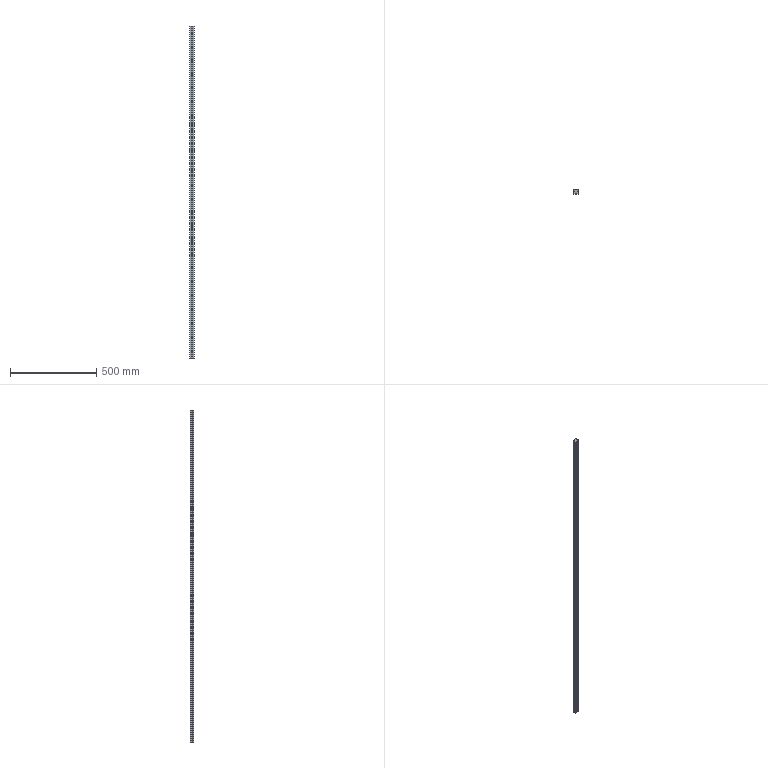Part | STEP file | HIWIN linear rail EGH30-1920-40-40 | 1 solid | 160 faces | box 28 x 23 x 1920 mm | volume 1071300 mm3 | cylinder 114 | plane 46 | commonest cylinder face diameters 7 x48 11 x48 0.6 x8 3 x6 5 x4